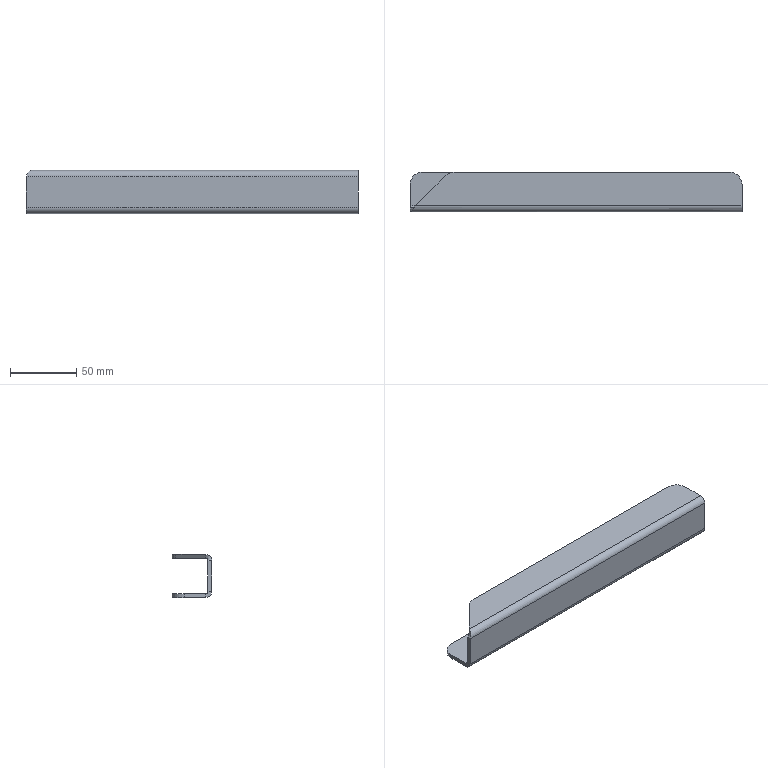Part | NX | features BREP 1 | 1 solid | 26 faces | box 250.19 x 29.972 x 32.487 mm | volume 61350 mm3 | plane 17 | cylinder 8 | spline 1 | commonest cylinder face diameters 19.05 x4 3.175 x2 9.169 x2
STEP:
#1=CARTESIAN_POINT('',(125.095,0.,11.659));
#2=VERTEX_POINT('',#1);
#3=CARTESIAN_POINT('',(125.095,0.,-11.659));
#4=VERTEX_POINT('',#3);
#5=CARTESIAN_POINT('',(125.095,0.,11.659));
#6=DIRECTION('',(0.,0.,-1.));
#7=VECTOR('',#6,1000.);
#8=LINE('',#5,#7);
#9=EDGE_CURVE('',#2,#4,#8,.T.);
#10=ORIENTED_EDGE('',*,*,#9,.T.);
#11=CARTESIAN_POINT('',(-125.095,0.,-11.659));
#12=VERTEX_POINT('',#11);
#13=CARTESIAN_POINT('',(125.095,0.,-11.659));
#14=DIRECTION('',(-1.,0.,0.));
#15=VECTOR('',#14,1000.);
#16=LINE('',#13,#15);
#17=EDGE_CURVE('',#4,#12,#16,.T.);
#18=ORIENTED_EDGE('',*,*,#17,.T.);
#19=CARTESIAN_POINT('',(-125.095,0.,11.659));
#20=VERTEX_POINT('',#19);
#21=CARTESIAN_POINT('',(-125.095,0.,-11.659));
#22=DIRECTION('',(0.,0.,1.));
#23=VECTOR('',#22,1000.);
#24=LINE('',#21,#23);
#25=EDGE_CURVE('',#12,#20,#24,.T.);
#26=ORIENTED_EDGE('',*,*,#25,.T.);
#27=CARTESIAN_POINT('',(-125.095,0.,11.659));
#28=DIRECTION('',(1.,0.,0.));
#29=VECTOR('',#28,1000.);
#30=LINE('',#27,#29);
#31=EDGE_CURVE('',#20,#2,#30,.T.);
#32=ORIENTED_EDGE('',*,*,#31,.T.);
#33=EDGE_LOOP('',(#10,#18,#26,#32));
#34=FACE_BOUND('',#33,.T.);
#35=CARTESIAN_POINT('',(0.,0.,0.));
#36=DIRECTION('',(0.,1.,0.));
#37=DIRECTION('',(1.,0.,0.));
#38=AXIS2_PLACEMENT_3D('',#35,#36,#37);
#39=PLANE('',#38);
#40=ADVANCED_FACE('',(#34),#39,.T.);
#41=CARTESIAN_POINT('',(125.095,1.587,13.246));
#42=VERTEX_POINT('',#41);
#43=CARTESIAN_POINT('',(125.095,1.587,11.659));
#44=DIRECTION('',(1.,0.,0.));
#45=DIRECTION('',(0.,0.,1.));
#46=AXIS2_PLACEMENT_3D('',#43,#44,#45);
#47=CIRCLE('',#46,1.587);
#48=EDGE_CURVE('',#42,#2,#47,.T.);
#49=ORIENTED_EDGE('',*,*,#48,.T.);
#50=ORIENTED_EDGE('',*,*,#31,.F.);
#51=CARTESIAN_POINT('',(-121.103,1.587,13.246));
#52=VERTEX_POINT('',#51);
#53=CARTESIAN_POINT('',(-125.095,0.,11.659));
#54=CARTESIAN_POINT('',(-123.764,0.,12.49));
#55=CARTESIAN_POINT('',(-122.434,0.7563,13.246));
#56=CARTESIAN_POINT('',(-121.103,1.587,13.246));
#57=B_SPLINE_CURVE_WITH_KNOTS('',3,(#53,#54,#55,#56),.UNSPECIFIED.,.F.,.F.,(4,4),(0.,1.),.UNSPECIFIED.);
#58=EDGE_CURVE('',#52,#20,#57,.F.);
#59=ORIENTED_EDGE('',*,*,#58,.F.);
#60=CARTESIAN_POINT('',(-121.103,1.587,13.246));
#61=DIRECTION('',(1.,0.,0.));
#62=VECTOR('',#61,1000.);
#63=LINE('',#60,#62);
#64=EDGE_CURVE('',#52,#42,#63,.T.);
#65=ORIENTED_EDGE('',*,*,#64,.T.);
#66=EDGE_LOOP('',(#49,#50,#59,#65));
#67=FACE_BOUND('',#66,.T.);
#68=CARTESIAN_POINT('',(-125.095,1.587,11.659));
#69=DIRECTION('',(1.,0.,0.));
#70=DIRECTION('',(0.,0.,1.));
#71=AXIS2_PLACEMENT_3D('',#68,#69,#70);
#72=CYLINDRICAL_SURFACE('',#71,1.587);
#73=ADVANCED_FACE('',(#67),#72,.F.);
#74=CARTESIAN_POINT('',(115.57,26.975,13.246));
#75=VERTEX_POINT('',#74);
#76=CARTESIAN_POINT('',(-91.77,26.975,13.246));
#77=VERTEX_POINT('',#76);
#78=CARTESIAN_POINT('',(115.57,26.975,13.246));
#79=DIRECTION('',(-1.,0.,0.));
#80=VECTOR('',#79,1000.);
#81=LINE('',#78,#80);
#82=EDGE_CURVE('',#75,#77,#81,.T.);
#83=ORIENTED_EDGE('',*,*,#82,.F.);
#84=CARTESIAN_POINT('',(125.095,17.45,13.246));
#85=VERTEX_POINT('',#84);
#86=CARTESIAN_POINT('',(115.57,17.45,13.246));
#87=DIRECTION('',(0.,0.,-1.));
#88=DIRECTION('',(0.,1.,0.));
#89=AXIS2_PLACEMENT_3D('',#86,#87,#88);
#90=CIRCLE('',#89,9.525);
#91=EDGE_CURVE('',#75,#85,#90,.T.);
#92=ORIENTED_EDGE('',*,*,#91,.T.);
#93=CARTESIAN_POINT('',(125.095,1.587,13.246));
#94=DIRECTION('',(0.,1.,0.));
#95=VECTOR('',#94,1000.);
#96=LINE('',#93,#95);
#97=EDGE_CURVE('',#42,#85,#96,.T.);
#98=ORIENTED_EDGE('',*,*,#97,.F.);
#99=ORIENTED_EDGE('',*,*,#64,.F.);
#100=CARTESIAN_POINT('',(-98.505,24.185,13.246));
#101=VERTEX_POINT('',#100);
#102=CARTESIAN_POINT('',(-121.103,1.587,13.246));
#103=DIRECTION('',(0.7071,0.7071,0.));
#104=VECTOR('',#103,1000.);
#105=LINE('',#102,#104);
#106=EDGE_CURVE('',#52,#101,#105,.T.);
#107=ORIENTED_EDGE('',*,*,#106,.T.);
#108=CARTESIAN_POINT('',(-91.77,17.45,13.246));
#109=DIRECTION('',(0.,0.,-1.));
#110=DIRECTION('',(-0.7071,0.7071,0.));
#111=AXIS2_PLACEMENT_3D('',#108,#109,#110);
#112=CIRCLE('',#111,9.525);
#113=EDGE_CURVE('',#101,#77,#112,.T.);
#114=ORIENTED_EDGE('',*,*,#113,.T.);
#115=EDGE_LOOP('',(#83,#92,#98,#99,#107,#114));
#116=FACE_BOUND('',#115,.T.);
#117=CARTESIAN_POINT('',(-65.65,0.,13.246));
#118=DIRECTION('',(0.,0.,1.));
#119=DIRECTION('',(1.,0.,0.));
#120=AXIS2_PLACEMENT_3D('',#117,#118,#119);
#121=PLANE('',#120);
#122=ADVANCED_FACE('',(#116),#121,.F.);
#123=CARTESIAN_POINT('',(-91.77,26.975,16.243));
#124=VERTEX_POINT('',#123);
#125=CARTESIAN_POINT('',(-98.505,24.185,16.243));
#126=VERTEX_POINT('',#125);
#127=CARTESIAN_POINT('',(-91.77,17.45,16.243));
#128=DIRECTION('',(0.,0.,1.));
#129=DIRECTION('',(0.,1.,0.));
#130=AXIS2_PLACEMENT_3D('',#127,#128,#129);
#131=CIRCLE('',#130,9.525);
#132=EDGE_CURVE('',#124,#126,#131,.T.);
#133=ORIENTED_EDGE('',*,*,#132,.F.);
#134=CARTESIAN_POINT('',(-91.77,26.975,16.243));
#135=DIRECTION('',(0.,0.,-1.));
#136=VECTOR('',#135,1000.);
#137=LINE('',#134,#136);
#138=EDGE_CURVE('',#124,#77,#137,.T.);
#139=ORIENTED_EDGE('',*,*,#138,.T.);
#140=ORIENTED_EDGE('',*,*,#113,.F.);
#141=CARTESIAN_POINT('',(-98.505,24.185,16.243));
#142=DIRECTION('',(0.,0.,-1.));
#143=VECTOR('',#142,1000.);
#144=LINE('',#141,#143);
#145=EDGE_CURVE('',#126,#101,#144,.T.);
#146=ORIENTED_EDGE('',*,*,#145,.F.);
#147=EDGE_LOOP('',(#133,#139,#140,#146));
#148=FACE_BOUND('',#147,.T.);
#149=CARTESIAN_POINT('',(-91.77,17.45,16.613));
#150=DIRECTION('',(0.,0.,-1.));
#151=DIRECTION('',(-0.7071,0.7071,0.));
#152=AXIS2_PLACEMENT_3D('',#149,#150,#151);
#153=CYLINDRICAL_SURFACE('',#152,9.525);
#154=ADVANCED_FACE('',(#148),#153,.T.);
#155=ORIENTED_EDGE('',*,*,#106,.F.);
#156=CARTESIAN_POINT('',(-121.103,1.587,16.243));
#157=VERTEX_POINT('',#156);
#158=CARTESIAN_POINT('',(-121.103,1.587,13.246));
#159=DIRECTION('',(0.,0.,1.));
#160=VECTOR('',#159,1000.);
#161=LINE('',#158,#160);
#162=EDGE_CURVE('',#52,#157,#161,.T.);
#163=ORIENTED_EDGE('',*,*,#162,.T.);
#164=CARTESIAN_POINT('',(-121.103,1.587,16.243));
#165=DIRECTION('',(0.7071,0.7071,0.));
#166=VECTOR('',#165,1000.);
#167=LINE('',#164,#166);
#168=EDGE_CURVE('',#157,#126,#167,.T.);
#169=ORIENTED_EDGE('',*,*,#168,.T.);
#170=ORIENTED_EDGE('',*,*,#145,.T.);
#171=EDGE_LOOP('',(#155,#163,#169,#170));
#172=FACE_BOUND('',#171,.T.);
#173=CARTESIAN_POINT('',(-108.409,14.281,14.745));
#174=DIRECTION('',(-0.7071,0.7071,0.));
#175=DIRECTION('',(0.,0.,1.));
#176=AXIS2_PLACEMENT_3D('',#173,#174,#175);
#177=PLANE('',#176);
#178=ADVANCED_FACE('',(#172),#177,.T.);
#179=ORIENTED_EDGE('',*,*,#168,.F.);
#180=CARTESIAN_POINT('',(125.095,1.587,16.243));
#181=VERTEX_POINT('',#180);
#182=CARTESIAN_POINT('',(-121.103,1.587,16.243));
#183=DIRECTION('',(1.,0.,0.));
#184=VECTOR('',#183,1000.);
#185=LINE('',#182,#184);
#186=EDGE_CURVE('',#157,#181,#185,.T.);
#187=ORIENTED_EDGE('',*,*,#186,.T.);
#188=CARTESIAN_POINT('',(125.095,17.45,16.243));
#189=VERTEX_POINT('',#188);
#190=CARTESIAN_POINT('',(125.095,1.587,16.243));
#191=DIRECTION('',(0.,1.,0.));
#192=VECTOR('',#191,1000.);
#193=LINE('',#190,#192);
#194=EDGE_CURVE('',#181,#189,#193,.T.);
#195=ORIENTED_EDGE('',*,*,#194,.T.);
#196=CARTESIAN_POINT('',(115.57,26.975,16.243));
#197=VERTEX_POINT('',#196);
#198=CARTESIAN_POINT('',(115.57,17.45,16.243));
#199=DIRECTION('',(0.,0.,1.));
#200=DIRECTION('',(1.,0.,0.));
#201=AXIS2_PLACEMENT_3D('',#198,#199,#200);
#202=CIRCLE('',#201,9.525);
#203=EDGE_CURVE('',#189,#197,#202,.T.);
#204=ORIENTED_EDGE('',*,*,#203,.T.);
#205=CARTESIAN_POINT('',(115.57,26.975,16.243));
#206=DIRECTION('',(-1.,0.,0.));
#207=VECTOR('',#206,1000.);
#208=LINE('',#205,#207);
#209=EDGE_CURVE('',#197,#124,#208,.T.);
#210=ORIENTED_EDGE('',*,*,#209,.T.);
#211=ORIENTED_EDGE('',*,*,#132,.T.);
#212=EDGE_LOOP('',(#179,#187,#195,#204,#210,#211));
#213=FACE_BOUND('',#212,.T.);
#214=CARTESIAN_POINT('',(-65.65,0.,16.243));
#215=DIRECTION('',(0.,0.,1.));
#216=DIRECTION('',(1.,0.,0.));
#217=AXIS2_PLACEMENT_3D('',#214,#215,#216);
#218=PLANE('',#217);
#219=ADVANCED_FACE('',(#213),#218,.T.);
#220=ORIENTED_EDGE('',*,*,#209,.F.);
#221=CARTESIAN_POINT('',(115.57,26.975,16.243));
#222=DIRECTION('',(0.,0.,-1.));
#223=VECTOR('',#222,1000.);
#224=LINE('',#221,#223);
#225=EDGE_CURVE('',#197,#75,#224,.T.);
#226=ORIENTED_EDGE('',*,*,#225,.T.);
#227=ORIENTED_EDGE('',*,*,#82,.T.);
#228=ORIENTED_EDGE('',*,*,#138,.F.);
#229=EDGE_LOOP('',(#220,#226,#227,#228));
#230=FACE_BOUND('',#229,.T.);
#231=CARTESIAN_POINT('',(0.,26.975,14.745));
#232=DIRECTION('',(0.,-1.,0.));
#233=DIRECTION('',(0.,0.,-1.));
#234=AXIS2_PLACEMENT_3D('',#231,#232,#233);
#235=PLANE('',#234);
#236=ADVANCED_FACE('',(#230),#235,.F.);
#237=ORIENTED_EDGE('',*,*,#203,.F.);
#238=CARTESIAN_POINT('',(125.095,17.45,16.243));
#239=DIRECTION('',(0.,0.,-1.));
#240=VECTOR('',#239,1000.);
#241=LINE('',#238,#240);
#242=EDGE_CURVE('',#189,#85,#241,.T.);
#243=ORIENTED_EDGE('',*,*,#242,.T.);
#244=ORIENTED_EDGE('',*,*,#91,.F.);
#245=ORIENTED_EDGE('',*,*,#225,.F.);
#246=EDGE_LOOP('',(#237,#243,#244,#245));
#247=FACE_BOUND('',#246,.T.);
#248=CARTESIAN_POINT('',(115.57,17.45,16.613));
#249=DIRECTION('',(0.,0.,-1.));
#250=DIRECTION('',(0.,1.,0.));
#251=AXIS2_PLACEMENT_3D('',#248,#249,#250);
#252=CYLINDRICAL_SURFACE('',#251,9.525);
#253=ADVANCED_FACE('',(#247),#252,.T.);
#254=ORIENTED_EDGE('',*,*,#194,.F.);
#255=CARTESIAN_POINT('',(125.095,1.587,13.246));
#256=DIRECTION('',(0.,0.,1.));
#257=VECTOR('',#256,1000.);
#258=LINE('',#255,#257);
#259=EDGE_CURVE('',#42,#181,#258,.T.);
#260=ORIENTED_EDGE('',*,*,#259,.F.);
#261=ORIENTED_EDGE('',*,*,#97,.T.);
#262=ORIENTED_EDGE('',*,*,#242,.F.);
#263=EDGE_LOOP('',(#254,#260,#261,#262));
#264=FACE_BOUND('',#263,.T.);
#265=CARTESIAN_POINT('',(125.095,14.281,14.745));
#266=DIRECTION('',(-1.,0.,0.));
#267=DIRECTION('',(0.,0.,1.));
#268=AXIS2_PLACEMENT_3D('',#265,#266,#267);
#269=PLANE('',#268);
#270=ADVANCED_FACE('',(#264),#269,.F.);
#271=ORIENTED_EDGE('',*,*,#259,.T.);
#272=CARTESIAN_POINT('',(125.095,-2.997,11.659));
#273=VERTEX_POINT('',#272);
#274=CARTESIAN_POINT('',(125.095,1.587,11.659));
#275=DIRECTION('',(1.,0.,0.));
#276=DIRECTION('',(0.,0.,1.));
#277=AXIS2_PLACEMENT_3D('',#274,#275,#276);
#278=CIRCLE('',#277,4.585);
#279=EDGE_CURVE('',#181,#273,#278,.T.);
#280=ORIENTED_EDGE('',*,*,#279,.T.);
#281=CARTESIAN_POINT('',(125.095,0.,11.659));
#282=DIRECTION('',(0.,-1.,0.));
#283=VECTOR('',#282,1000.);
#284=LINE('',#281,#283);
#285=EDGE_CURVE('',#2,#273,#284,.T.);
#286=ORIENTED_EDGE('',*,*,#285,.F.);
#287=ORIENTED_EDGE('',*,*,#48,.F.);
#288=EDGE_LOOP('',(#271,#280,#286,#287));
#289=FACE_BOUND('',#288,.T.);
#290=CARTESIAN_POINT('',(125.095,-0.5947,13.841));
#291=DIRECTION('',(1.,0.,0.));
#292=DIRECTION('',(0.,0.,-1.));
#293=AXIS2_PLACEMENT_3D('',#290,#291,#292);
#294=PLANE('',#293);
#295=ADVANCED_FACE('',(#289),#294,.T.);
#296=ORIENTED_EDGE('',*,*,#285,.T.);
#297=CARTESIAN_POINT('',(125.095,-2.997,-11.659));
#298=VERTEX_POINT('',#297);
#299=CARTESIAN_POINT('',(125.095,-2.997,11.659));
#300=DIRECTION('',(0.,0.,-1.));
#301=VECTOR('',#300,1000.);
#302=LINE('',#299,#301);
#303=EDGE_CURVE('',#273,#298,#302,.T.);
#304=ORIENTED_EDGE('',*,*,#303,.T.);
#305=CARTESIAN_POINT('',(125.095,0.,-11.659));
#306=DIRECTION('',(0.,-1.,0.));
#307=VECTOR('',#306,1000.);
#308=LINE('',#305,#307);
#309=EDGE_CURVE('',#4,#298,#308,.T.);
#310=ORIENTED_EDGE('',*,*,#309,.F.);
#311=ORIENTED_EDGE('',*,*,#9,.F.);
#312=EDGE_LOOP('',(#296,#304,#310,#311));
#313=FACE_BOUND('',#312,.T.);
#314=CARTESIAN_POINT('',(125.095,-1.499,0.));
#315=DIRECTION('',(1.,0.,0.));
#316=DIRECTION('',(0.,1.,0.));
#317=AXIS2_PLACEMENT_3D('',#314,#315,#316);
#318=PLANE('',#317);
#319=ADVANCED_FACE('',(#313),#318,.T.);
#320=ORIENTED_EDGE('',*,*,#309,.T.);
#321=CARTESIAN_POINT('',(125.095,1.587,-16.243));
#322=VERTEX_POINT('',#321);
#323=CARTESIAN_POINT('',(125.095,1.587,-11.659));
#324=DIRECTION('',(-1.,0.,0.));
#325=DIRECTION('',(0.,0.,-1.));
#326=AXIS2_PLACEMENT_3D('',#323,#324,#325);
#327=CIRCLE('',#326,4.585);
#328=EDGE_CURVE('',#322,#298,#327,.T.);
#329=ORIENTED_EDGE('',*,*,#328,.F.);
#330=CARTESIAN_POINT('',(125.095,1.587,-13.246));
#331=VERTEX_POINT('',#330);
#332=CARTESIAN_POINT('',(125.095,1.587,-13.246));
#333=DIRECTION('',(0.,0.,-1.));
#334=VECTOR('',#333,1000.);
#335=LINE('',#332,#334);
#336=EDGE_CURVE('',#331,#322,#335,.T.);
#337=ORIENTED_EDGE('',*,*,#336,.F.);
#338=CARTESIAN_POINT('',(125.095,1.587,-11.659));
#339=DIRECTION('',(-1.,0.,0.));
#340=DIRECTION('',(0.,0.,-1.));
#341=AXIS2_PLACEMENT_3D('',#338,#339,#340);
#342=CIRCLE('',#341,1.587);
#343=EDGE_CURVE('',#331,#4,#342,.T.);
#344=ORIENTED_EDGE('',*,*,#343,.T.);
#345=EDGE_LOOP('',(#320,#329,#337,#344));
#346=FACE_BOUND('',#345,.T.);
#347=CARTESIAN_POINT('',(125.095,-0.5947,-13.841));
#348=DIRECTION('',(-1.,0.,0.));
#349=DIRECTION('',(0.,0.,1.));
#350=AXIS2_PLACEMENT_3D('',#347,#348,#349);
#351=PLANE('',#350);
#352=ADVANCED_FACE('',(#346),#351,.F.);
#353=CARTESIAN_POINT('',(-125.095,1.587,-13.246));
#354=VERTEX_POINT('',#353);
#355=CARTESIAN_POINT('',(-125.095,1.587,-11.659));
#356=DIRECTION('',(-1.,0.,0.));
#357=DIRECTION('',(0.,0.,-1.));
#358=AXIS2_PLACEMENT_3D('',#355,#356,#357);
#359=CIRCLE('',#358,1.587);
#360=EDGE_CURVE('',#354,#12,#359,.T.);
#361=ORIENTED_EDGE('',*,*,#360,.T.);
#362=ORIENTED_EDGE('',*,*,#17,.F.);
#363=ORIENTED_EDGE('',*,*,#343,.F.);
#364=CARTESIAN_POINT('',(125.095,1.587,-13.246));
#365=DIRECTION('',(-1.,0.,0.));
#366=VECTOR('',#365,1000.);
#367=LINE('',#364,#366);
#368=EDGE_CURVE('',#331,#354,#367,.T.);
#369=ORIENTED_EDGE('',*,*,#368,.T.);
#370=EDGE_LOOP('',(#361,#362,#363,#369));
#371=FACE_BOUND('',#370,.T.);
#372=CARTESIAN_POINT('',(125.095,1.587,-11.659));
#373=DIRECTION('',(-1.,0.,0.));
#374=DIRECTION('',(0.,0.,-1.));
#375=AXIS2_PLACEMENT_3D('',#372,#373,#374);
#376=CYLINDRICAL_SURFACE('',#375,1.587);
#377=ADVANCED_FACE('',(#371),#376,.F.);
#378=CARTESIAN_POINT('',(-115.57,26.975,-13.246));
#379=VERTEX_POINT('',#378);
#380=CARTESIAN_POINT('',(115.57,26.975,-13.246));
#381=VERTEX_POINT('',#380);
#382=CARTESIAN_POINT('',(-115.57,26.975,-13.246));
#383=DIRECTION('',(1.,0.,0.));
#384=VECTOR('',#383,1000.);
#385=LINE('',#382,#384);
#386=EDGE_CURVE('',#379,#381,#385,.T.);
#387=ORIENTED_EDGE('',*,*,#386,.F.);
#388=CARTESIAN_POINT('',(-125.095,17.45,-13.246));
#389=VERTEX_POINT('',#388);
#390=CARTESIAN_POINT('',(-115.57,17.45,-13.246));
#391=DIRECTION('',(0.,0.,1.));
#392=DIRECTION('',(0.,1.,0.));
#393=AXIS2_PLACEMENT_3D('',#390,#391,#392);
#394=CIRCLE('',#393,9.525);
#395=EDGE_CURVE('',#379,#389,#394,.T.);
#396=ORIENTED_EDGE('',*,*,#395,.T.);
#397=CARTESIAN_POINT('',(-125.095,1.587,-13.246));
#398=DIRECTION('',(0.,1.,0.));
#399=VECTOR('',#398,1000.);
#400=LINE('',#397,#399);
#401=EDGE_CURVE('',#354,#389,#400,.T.);
#402=ORIENTED_EDGE('',*,*,#401,.F.);
#403=ORIENTED_EDGE('',*,*,#368,.F.);
#404=CARTESIAN_POINT('',(125.095,17.45,-13.246));
#405=VERTEX_POINT('',#404);
#406=CARTESIAN_POINT('',(125.095,17.45,-13.246));
#407=DIRECTION('',(0.,-1.,0.));
#408=VECTOR('',#407,1000.);
#409=LINE('',#406,#408);
#410=EDGE_CURVE('',#405,#331,#409,.T.);
#411=ORIENTED_EDGE('',*,*,#410,.F.);
#412=CARTESIAN_POINT('',(115.57,17.45,-13.246));
#413=DIRECTION('',(0.,0.,1.));
#414=DIRECTION('',(1.,0.,0.));
#415=AXIS2_PLACEMENT_3D('',#412,#413,#414);
#416=CIRCLE('',#415,9.525);
#417=EDGE_CURVE('',#405,#381,#416,.T.);
#418=ORIENTED_EDGE('',*,*,#417,.T.);
#419=EDGE_LOOP('',(#387,#396,#402,#403,#411,#418));
#420=FACE_BOUND('',#419,.T.);
#421=CARTESIAN_POINT('',(65.65,0.,-13.246));
#422=DIRECTION('',(0.,0.,-1.));
#423=DIRECTION('',(0.,-1.,0.));
#424=AXIS2_PLACEMENT_3D('',#421,#422,#423);
#425=PLANE('',#424);
#426=ADVANCED_FACE('',(#420),#425,.F.);
#427=CARTESIAN_POINT('',(115.57,26.975,-16.243));
#428=VERTEX_POINT('',#427);
#429=CARTESIAN_POINT('',(125.095,17.45,-16.243));
#430=VERTEX_POINT('',#429);
#431=CARTESIAN_POINT('',(115.57,17.45,-16.243));
#432=DIRECTION('',(0.,0.,-1.));
#433=DIRECTION('',(0.,1.,0.));
#434=AXIS2_PLACEMENT_3D('',#431,#432,#433);
#435=CIRCLE('',#434,9.525);
#436=EDGE_CURVE('',#428,#430,#435,.T.);
#437=ORIENTED_EDGE('',*,*,#436,.F.);
#438=CARTESIAN_POINT('',(115.57,26.975,-16.243));
#439=DIRECTION('',(0.,0.,1.));
#440=VECTOR('',#439,1000.);
#441=LINE('',#438,#440);
#442=EDGE_CURVE('',#428,#381,#441,.T.);
#443=ORIENTED_EDGE('',*,*,#442,.T.);
#444=ORIENTED_EDGE('',*,*,#417,.F.);
#445=CARTESIAN_POINT('',(125.095,17.45,-16.243));
#446=DIRECTION('',(0.,0.,1.));
#447=VECTOR('',#446,1000.);
#448=LINE('',#445,#447);
#449=EDGE_CURVE('',#430,#405,#448,.T.);
#450=ORIENTED_EDGE('',*,*,#449,.F.);
#451=EDGE_LOOP('',(#437,#443,#444,#450));
#452=FACE_BOUND('',#451,.T.);
#453=CARTESIAN_POINT('',(115.57,17.45,-16.613));
#454=DIRECTION('',(0.,0.,1.));
#455=DIRECTION('',(1.,0.,0.));
#456=AXIS2_PLACEMENT_3D('',#453,#454,#455);
#457=CYLINDRICAL_SURFACE('',#456,9.525);
#458=ADVANCED_FACE('',(#452),#457,.T.);
#459=ORIENTED_EDGE('',*,*,#410,.T.);
#460=ORIENTED_EDGE('',*,*,#336,.T.);
#461=CARTESIAN_POINT('',(125.095,17.45,-16.243));
#462=DIRECTION('',(0.,-1.,0.));
#463=VECTOR('',#462,1000.);
#464=LINE('',#461,#463);
#465=EDGE_CURVE('',#430,#322,#464,.T.);
#466=ORIENTED_EDGE('',*,*,#465,.F.);
#467=ORIENTED_EDGE('',*,*,#449,.T.);
#468=EDGE_LOOP('',(#459,#460,#466,#467));
#469=FACE_BOUND('',#468,.T.);
#470=CARTESIAN_POINT('',(125.095,14.281,-14.745));
#471=DIRECTION('',(-1.,0.,0.));
#472=DIRECTION('',(0.,0.,1.));
#473=AXIS2_PLACEMENT_3D('',#470,#471,#472);
#474=PLANE('',#473);
#475=ADVANCED_FACE('',(#469),#474,.F.);
#476=ORIENTED_EDGE('',*,*,#465,.T.);
#477=CARTESIAN_POINT('',(-125.095,1.587,-16.243));
#478=VERTEX_POINT('',#477);
#479=CARTESIAN_POINT('',(125.095,1.587,-16.243));
#480=DIRECTION('',(-1.,0.,0.));
#481=VECTOR('',#480,1000.);
#482=LINE('',#479,#481);
#483=EDGE_CURVE('',#322,#478,#482,.T.);
#484=ORIENTED_EDGE('',*,*,#483,.T.);
#485=CARTESIAN_POINT('',(-125.095,17.45,-16.243));
#486=VERTEX_POINT('',#485);
#487=CARTESIAN_POINT('',(-125.095,1.587,-16.243));
#488=DIRECTION('',(0.,1.,0.));
#489=VECTOR('',#488,1000.);
#490=LINE('',#487,#489);
#491=EDGE_CURVE('',#478,#486,#490,.T.);
#492=ORIENTED_EDGE('',*,*,#491,.T.);
#493=CARTESIAN_POINT('',(-115.57,26.975,-16.243));
#494=VERTEX_POINT('',#493);
#495=CARTESIAN_POINT('',(-115.57,17.45,-16.243));
#496=DIRECTION('',(0.,0.,-1.));
#497=DIRECTION('',(-1.,0.,0.));
#498=AXIS2_PLACEMENT_3D('',#495,#496,#497);
#499=CIRCLE('',#498,9.525);
#500=EDGE_CURVE('',#486,#494,#499,.T.);
#501=ORIENTED_EDGE('',*,*,#500,.T.);
#502=CARTESIAN_POINT('',(-115.57,26.975,-16.243));
#503=DIRECTION('',(1.,0.,0.));
#504=VECTOR('',#503,1000.);
#505=LINE('',#502,#504);
#506=EDGE_CURVE('',#494,#428,#505,.T.);
#507=ORIENTED_EDGE('',*,*,#506,.T.);
#508=ORIENTED_EDGE('',*,*,#436,.T.);
#509=EDGE_LOOP('',(#476,#484,#492,#501,#507,#508));
#510=FACE_BOUND('',#509,.T.);
#511=CARTESIAN_POINT('',(65.65,0.,-16.243));
#512=DIRECTION('',(0.,0.,-1.));
#513=DIRECTION('',(0.,-1.,0.));
#514=AXIS2_PLACEMENT_3D('',#511,#512,#513);
#515=PLANE('',#514);
#516=ADVANCED_FACE('',(#510),#515,.T.);
#517=ORIENTED_EDGE('',*,*,#506,.F.);
#518=CARTESIAN_POINT('',(-115.57,26.975,-16.243));
#519=DIRECTION('',(0.,0.,1.));
#520=VECTOR('',#519,1000.);
#521=LINE('',#518,#520);
#522=EDGE_CURVE('',#494,#379,#521,.T.);
#523=ORIENTED_EDGE('',*,*,#522,.T.);
#524=ORIENTED_EDGE('',*,*,#386,.T.);
#525=ORIENTED_EDGE('',*,*,#442,.F.);
#526=EDGE_LOOP('',(#517,#523,#524,#525));
#527=FACE_BOUND('',#526,.T.);
#528=CARTESIAN_POINT('',(0.,26.975,-14.745));
#529=DIRECTION('',(0.,-1.,0.));
#530=DIRECTION('',(0.,0.,-1.));
#531=AXIS2_PLACEMENT_3D('',#528,#529,#530);
#532=PLANE('',#531);
#533=ADVANCED_FACE('',(#527),#532,.F.);
#534=ORIENTED_EDGE('',*,*,#500,.F.);
#535=CARTESIAN_POINT('',(-125.095,17.45,-16.243));
#536=DIRECTION('',(0.,0.,1.));
#537=VECTOR('',#536,1000.);
#538=LINE('',#535,#537);
#539=EDGE_CURVE('',#486,#389,#538,.T.);
#540=ORIENTED_EDGE('',*,*,#539,.T.);
#541=ORIENTED_EDGE('',*,*,#395,.F.);
#542=ORIENTED_EDGE('',*,*,#522,.F.);
#543=EDGE_LOOP('',(#534,#540,#541,#542));
#544=FACE_BOUND('',#543,.T.);
#545=CARTESIAN_POINT('',(-115.57,17.45,-16.613));
#546=DIRECTION('',(0.,0.,1.));
#547=DIRECTION('',(0.,1.,0.));
#548=AXIS2_PLACEMENT_3D('',#545,#546,#547);
#549=CYLINDRICAL_SURFACE('',#548,9.525);
#550=ADVANCED_FACE('',(#544),#549,.T.);
#551=ORIENTED_EDGE('',*,*,#491,.F.);
#552=CARTESIAN_POINT('',(-125.095,1.587,-13.246));
#553=DIRECTION('',(0.,0.,-1.));
#554=VECTOR('',#553,1000.);
#555=LINE('',#552,#554);
#556=EDGE_CURVE('',#354,#478,#555,.T.);
#557=ORIENTED_EDGE('',*,*,#556,.F.);
#558=ORIENTED_EDGE('',*,*,#401,.T.);
#559=ORIENTED_EDGE('',*,*,#539,.F.);
#560=EDGE_LOOP('',(#551,#557,#558,#559));
#561=FACE_BOUND('',#560,.T.);
#562=CARTESIAN_POINT('',(-125.095,14.281,-14.745));
#563=DIRECTION('',(1.,0.,0.));
#564=DIRECTION('',(0.,1.,0.));
#565=AXIS2_PLACEMENT_3D('',#562,#563,#564);
#566=PLANE('',#565);
#567=ADVANCED_FACE('',(#561),#566,.F.);
#568=ORIENTED_EDGE('',*,*,#556,.T.);
#569=CARTESIAN_POINT('',(-125.095,-2.997,-11.659));
#570=VERTEX_POINT('',#569);
#571=CARTESIAN_POINT('',(-125.095,1.587,-11.659));
#572=DIRECTION('',(-1.,0.,0.));
#573=DIRECTION('',(0.,0.,-1.));
#574=AXIS2_PLACEMENT_3D('',#571,#572,#573);
#575=CIRCLE('',#574,4.585);
#576=EDGE_CURVE('',#478,#570,#575,.T.);
#577=ORIENTED_EDGE('',*,*,#576,.T.);
#578=CARTESIAN_POINT('',(-125.095,0.,-11.659));
#579=DIRECTION('',(0.,-1.,0.));
#580=VECTOR('',#579,1000.);
#581=LINE('',#578,#580);
#582=EDGE_CURVE('',#12,#570,#581,.T.);
#583=ORIENTED_EDGE('',*,*,#582,.F.);
#584=ORIENTED_EDGE('',*,*,#360,.F.);
#585=EDGE_LOOP('',(#568,#577,#583,#584));
#586=FACE_BOUND('',#585,.T.);
#587=CARTESIAN_POINT('',(-125.095,-0.5947,-13.841));
#588=DIRECTION('',(-1.,0.,0.));
#589=DIRECTION('',(0.,0.,1.));
#590=AXIS2_PLACEMENT_3D('',#587,#588,#589);
#591=PLANE('',#590);
#592=ADVANCED_FACE('',(#586),#591,.T.);
#593=ORIENTED_EDGE('',*,*,#582,.T.);
#594=CARTESIAN_POINT('',(-125.095,-2.997,11.659));
#595=VERTEX_POINT('',#594);
#596=CARTESIAN_POINT('',(-125.095,-2.997,-11.659));
#597=DIRECTION('',(0.,0.,1.));
#598=VECTOR('',#597,1000.);
#599=LINE('',#596,#598);
#600=EDGE_CURVE('',#570,#595,#599,.T.);
#601=ORIENTED_EDGE('',*,*,#600,.T.);
#602=CARTESIAN_POINT('',(-125.095,0.,11.659));
#603=DIRECTION('',(0.,-1.,0.));
#604=VECTOR('',#603,1000.);
#605=LINE('',#602,#604);
#606=EDGE_CURVE('',#20,#595,#605,.T.);
#607=ORIENTED_EDGE('',*,*,#606,.F.);
#608=ORIENTED_EDGE('',*,*,#25,.F.);
#609=EDGE_LOOP('',(#593,#601,#607,#608));
#610=FACE_BOUND('',#609,.T.);
#611=CARTESIAN_POINT('',(-125.095,-1.499,0.));
#612=DIRECTION('',(-1.,0.,0.));
#613=DIRECTION('',(0.,0.,1.));
#614=AXIS2_PLACEMENT_3D('',#611,#612,#613);
#615=PLANE('',#614);
#616=ADVANCED_FACE('',(#610),#615,.T.);
#617=ORIENTED_EDGE('',*,*,#606,.T.);
#618=CARTESIAN_POINT('',(-121.103,1.587,16.243));
#619=CARTESIAN_POINT('',(-121.768,0.3872,16.243));
#620=CARTESIAN_POINT('',(-123.099,-2.004,15.25));
#621=CARTESIAN_POINT('',(-124.43,-2.997,12.859));
#622=CARTESIAN_POINT('',(-125.095,-2.997,11.659));
#623=B_SPLINE_CURVE_WITH_KNOTS('',3,(#618,#619,#620,#621,#622),.UNSPECIFIED.,.F.,.F.,(4,1,4),(0.,0.5,1.),.UNSPECIFIED.);
#624=EDGE_CURVE('',#157,#595,#623,.T.);
#625=ORIENTED_EDGE('',*,*,#624,.F.);
#626=ORIENTED_EDGE('',*,*,#162,.F.);
#627=ORIENTED_EDGE('',*,*,#58,.T.);
#628=EDGE_LOOP('',(#617,#625,#626,#627));
#629=FACE_BOUND('',#628,.T.);
#630=CARTESIAN_POINT('',(-125.236,0.3342,11.589));
#631=CARTESIAN_POINT('',(-125.236,-0.8845,11.521));
#632=CARTESIAN_POINT('',(-125.236,-2.103,11.454));
#633=CARTESIAN_POINT('',(-125.236,-3.322,11.386));
#634=CARTESIAN_POINT('',(-125.189,0.3328,11.612));
#635=CARTESIAN_POINT('',(-125.189,-0.8872,11.567));
#636=CARTESIAN_POINT('',(-125.189,-2.107,11.522));
#637=CARTESIAN_POINT('',(-125.189,-3.327,11.477));
#638=CARTESIAN_POINT('',(-124.809,0.3272,11.8));
#639=CARTESIAN_POINT('',(-124.809,-0.8977,11.937));
#640=CARTESIAN_POINT('',(-124.809,-2.123,12.074));
#641=CARTESIAN_POINT('',(-124.809,-3.348,12.211));
#642=CARTESIAN_POINT('',(-124.097,0.4012,12.151));
#643=CARTESIAN_POINT('',(-124.097,-0.7572,12.63));
#644=CARTESIAN_POINT('',(-124.097,-1.916,13.11));
#645=CARTESIAN_POINT('',(-124.097,-3.074,13.589));
#646=CARTESIAN_POINT('',(-123.099,0.6756,12.571));
#647=CARTESIAN_POINT('',(-123.099,-0.2096,13.456));
#648=CARTESIAN_POINT('',(-123.099,-1.095,14.341));
#649=CARTESIAN_POINT('',(-123.099,-1.98,15.226));
#650=CARTESIAN_POINT('',(-122.101,1.095,12.845));
#651=CARTESIAN_POINT('',(-122.101,0.6159,14.003));
#652=CARTESIAN_POINT('',(-122.101,0.1363,15.162));
#653=CARTESIAN_POINT('',(-122.101,-0.3432,16.32));
#654=CARTESIAN_POINT('',(-121.388,1.446,12.919));
#655=CARTESIAN_POINT('',(-121.388,1.309,14.144));
#656=CARTESIAN_POINT('',(-121.388,1.172,15.369));
#657=CARTESIAN_POINT('',(-121.388,1.035,16.594));
#658=CARTESIAN_POINT('',(-121.009,1.634,12.913));
#659=CARTESIAN_POINT('',(-121.009,1.679,14.133));
#660=CARTESIAN_POINT('',(-121.009,1.724,15.353));
#661=CARTESIAN_POINT('',(-121.009,1.769,16.573));
#662=CARTESIAN_POINT('',(-120.962,1.657,12.912));
#663=CARTESIAN_POINT('',(-120.962,1.725,14.131));
#664=CARTESIAN_POINT('',(-120.962,1.792,15.349));
#665=CARTESIAN_POINT('',(-120.962,1.86,16.568));
#666=B_SPLINE_SURFACE_WITH_KNOTS('',3,3,((#630,#631,#632,#633),(#634,#635,#636,#637),(#638,#639,#640,#641),(#642,#643,#644,#645),(#646,#647,#648,#649),(#650,#651,#652,#653),(#654,#655,#656,#657),(#658,#659,#660,#661),(#662,#663,#664,#665)),.RULED_SURF.,.F.,.F.,.F.,(4,1,1,1,1,1,4),(4,4),(-0.03527,0.,0.25,0.5,0.75,1.,1.035),(-0.1108,1.111),.UNSPECIFIED.);
#667=ADVANCED_FACE('',(#629),#666,.F.);
#668=ORIENTED_EDGE('',*,*,#624,.T.);
#669=CARTESIAN_POINT('',(-125.095,-2.997,11.659));
#670=DIRECTION('',(1.,0.,0.));
#671=VECTOR('',#670,1000.);
#672=LINE('',#669,#671);
#673=EDGE_CURVE('',#595,#273,#672,.T.);
#674=ORIENTED_EDGE('',*,*,#673,.T.);
#675=ORIENTED_EDGE('',*,*,#279,.F.);
#676=ORIENTED_EDGE('',*,*,#186,.F.);
#677=EDGE_LOOP('',(#668,#674,#675,#676));
#678=FACE_BOUND('',#677,.T.);
#679=CARTESIAN_POINT('',(-125.095,1.587,11.659));
#680=DIRECTION('',(1.,0.,0.));
#681=DIRECTION('',(0.,0.,1.));
#682=AXIS2_PLACEMENT_3D('',#679,#680,#681);
#683=CYLINDRICAL_SURFACE('',#682,4.585);
#684=ADVANCED_FACE('',(#678),#683,.T.);
#685=ORIENTED_EDGE('',*,*,#600,.F.);
#686=CARTESIAN_POINT('',(125.095,-2.997,-11.659));
#687=DIRECTION('',(-1.,0.,0.));
#688=VECTOR('',#687,1000.);
#689=LINE('',#686,#688);
#690=EDGE_CURVE('',#298,#570,#689,.T.);
#691=ORIENTED_EDGE('',*,*,#690,.F.);
#692=ORIENTED_EDGE('',*,*,#303,.F.);
#693=ORIENTED_EDGE('',*,*,#673,.F.);
#694=EDGE_LOOP('',(#685,#691,#692,#693));
#695=FACE_BOUND('',#694,.T.);
#696=CARTESIAN_POINT('',(0.,-2.997,0.));
#697=DIRECTION('',(0.,1.,0.));
#698=DIRECTION('',(1.,0.,0.));
#699=AXIS2_PLACEMENT_3D('',#696,#697,#698);
#700=PLANE('',#699);
#701=ADVANCED_FACE('',(#695),#700,.F.);
#702=ORIENTED_EDGE('',*,*,#328,.T.);
#703=ORIENTED_EDGE('',*,*,#690,.T.);
#704=ORIENTED_EDGE('',*,*,#576,.F.);
#705=ORIENTED_EDGE('',*,*,#483,.F.);
#706=EDGE_LOOP('',(#702,#703,#704,#705));
#707=FACE_BOUND('',#706,.T.);
#708=CARTESIAN_POINT('',(125.095,1.587,-11.659));
#709=DIRECTION('',(-1.,0.,0.));
#710=DIRECTION('',(0.,0.,-1.));
#711=AXIS2_PLACEMENT_3D('',#708,#709,#710);
#712=CYLINDRICAL_SURFACE('',#711,4.585);
#713=ADVANCED_FACE('',(#707),#712,.T.);
#714=CLOSED_SHELL('',(#40,#73,#122,#154,#178,#219,#236,#253,#270,#295,#319,#352,#377,#426,#458,#475,#516,#533,#550,#567,#592,#616,#667,#684,#701,#713));
#715=MANIFOLD_SOLID_BREP('',#714);
#716=(LENGTH_UNIT()NAMED_UNIT(*)SI_UNIT(.MILLI.,.METRE.));
#717=UNCERTAINTY_MEASURE_WITH_UNIT(LENGTH_MEASURE(0.0508),#716,'','');
#718=(NAMED_UNIT(*)PLANE_ANGLE_UNIT()SI_UNIT($,.RADIAN.));
#719=(NAMED_UNIT(*)SI_UNIT($,.STERADIAN.)SOLID_ANGLE_UNIT());
#720=(GEOMETRIC_REPRESENTATION_CONTEXT(3)GLOBAL_UNCERTAINTY_ASSIGNED_CONTEXT((#717))GLOBAL_UNIT_ASSIGNED_CONTEXT((#716,#718,#719))REPRESENTATION_CONTEXT('',''));
#721=ADVANCED_BREP_SHAPE_REPRESENTATION('',(#715),#720);